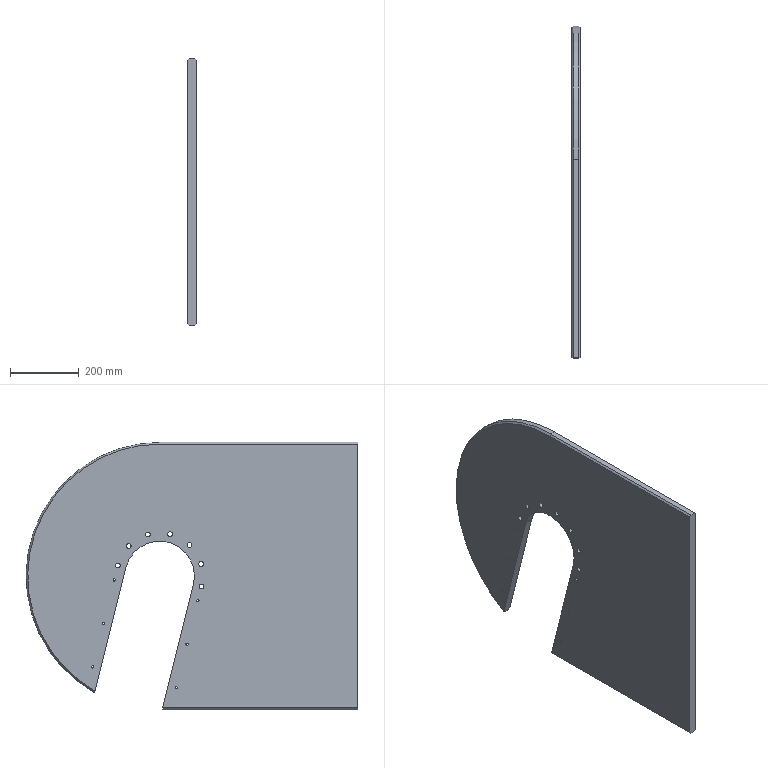Part | SolidWorks | features 3DProfileFeature 2, HoleWzd 2, Chamfer 1, CirPattern 1, Extrusion 1, ICE 1, LPattern 1, MirrorPattern 1 | 1 solid | 67 faces | box 25 x 962.5 x 775 mm | volume 14615637 mm3 | cone 28 | cylinder 28 | plane 11 | commonest cylinder face diameters 14 x14 6.8 x12 202 x1 775 x1